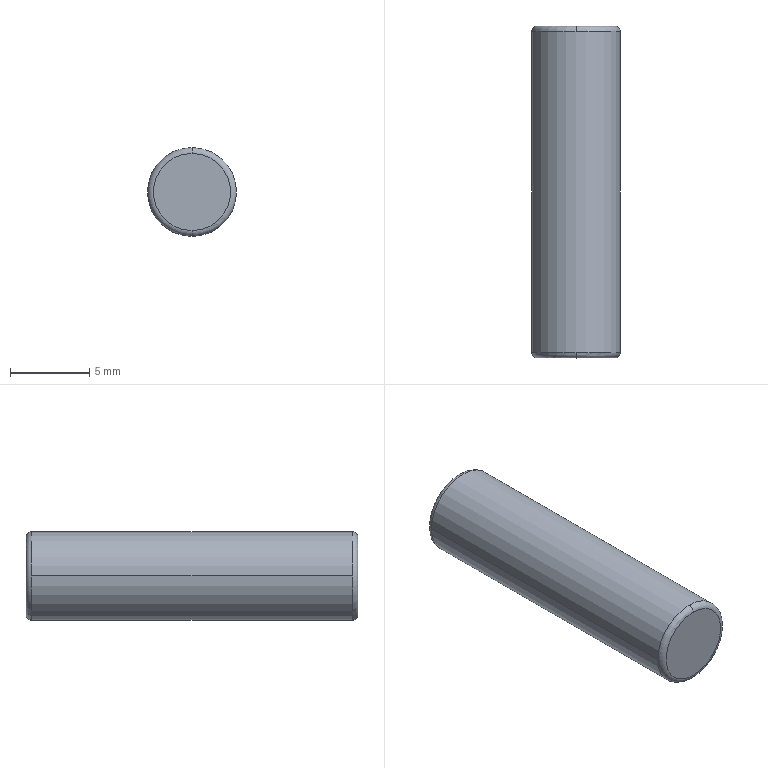Part | SolidWorks | features BaseBody 1 | 1 solid | 8 faces | box 5.625 x 21 x 5.625 mm | volume 520.859 mm3 | torus 4 | plane 2 | cylinder 2 | commonest cylinder face diameters 5.625 x2
STEP:
#1=CARTESIAN_POINT('',(-2092.012,757.069,-1580.068));
#2=VERTEX_POINT('',#1);
#3=CARTESIAN_POINT('',(-2092.012,757.069,-1575.181));
#4=VERTEX_POINT('',#3);
#5=CARTESIAN_POINT('',(-2092.012,757.069,-1577.624));
#6=DIRECTION('',(0.,-1.,0.));
#7=DIRECTION('',(1.,0.,0.));
#8=AXIS2_PLACEMENT_3D('',#5,#6,#7);
#9=CIRCLE('',#8,2.444);
#10=EDGE_CURVE('',#2,#4,#9,.T.);
#11=ORIENTED_EDGE('',*,*,#10,.T.);
#12=CARTESIAN_POINT('',(-2092.012,757.069,-1577.624));
#13=DIRECTION('',(0.,-1.,0.));
#14=DIRECTION('',(0.,0.,1.));
#15=AXIS2_PLACEMENT_3D('',#12,#13,#14);
#16=CIRCLE('',#15,2.444);
#17=EDGE_CURVE('',#4,#2,#16,.T.);
#18=ORIENTED_EDGE('',*,*,#17,.T.);
#19=EDGE_LOOP('',(#11,#18));
#20=FACE_OUTER_BOUND('',#19,.T.);
#21=CARTESIAN_POINT('',(-2094.675,757.069,-1580.313));
#22=DIRECTION('',(0.,-1.,0.));
#23=DIRECTION('',(0.,0.,-1.));
#24=AXIS2_PLACEMENT_3D('',#21,#22,#23);
#25=PLANE('',#24);
#26=ADVANCED_FACE('',(#20),#25,.T.);
#27=CARTESIAN_POINT('',(-2092.012,757.437,-1580.437));
#28=VERTEX_POINT('',#27);
#29=CARTESIAN_POINT('',(-2092.012,757.437,-1580.068));
#30=DIRECTION('',(-1.,0.,0.));
#31=DIRECTION('',(0.,0.,-1.));
#32=AXIS2_PLACEMENT_3D('',#29,#30,#31);
#33=CIRCLE('',#32,0.3687);
#34=EDGE_CURVE('',#28,#2,#33,.T.);
#35=ORIENTED_EDGE('',*,*,#34,.T.);
#36=ORIENTED_EDGE('',*,*,#17,.F.);
#37=CARTESIAN_POINT('',(-2092.012,757.437,-1574.812));
#38=VERTEX_POINT('',#37);
#39=CARTESIAN_POINT('',(-2092.012,757.437,-1575.181));
#40=DIRECTION('',(-1.,0.,0.));
#41=DIRECTION('',(0.,-1.,0.));
#42=AXIS2_PLACEMENT_3D('',#39,#40,#41);
#43=CIRCLE('',#42,0.3687);
#44=EDGE_CURVE('',#4,#38,#43,.T.);
#45=ORIENTED_EDGE('',*,*,#44,.T.);
#46=CARTESIAN_POINT('',(-2094.825,757.437,-1577.624));
#47=VERTEX_POINT('',#46);
#48=CARTESIAN_POINT('',(-2092.012,757.437,-1577.624));
#49=DIRECTION('',(0.,-1.,0.));
#50=DIRECTION('',(0.,0.,1.));
#51=AXIS2_PLACEMENT_3D('',#48,#49,#50);
#52=CIRCLE('',#51,2.813);
#53=EDGE_CURVE('',#38,#47,#52,.T.);
#54=ORIENTED_EDGE('',*,*,#53,.T.);
#55=CARTESIAN_POINT('',(-2092.012,757.437,-1577.624));
#56=DIRECTION('',(0.,-1.,0.));
#57=DIRECTION('',(-1.,0.,0.));
#58=AXIS2_PLACEMENT_3D('',#55,#56,#57);
#59=CIRCLE('',#58,2.813);
#60=EDGE_CURVE('',#47,#28,#59,.T.);
#61=ORIENTED_EDGE('',*,*,#60,.T.);
#62=EDGE_LOOP('',(#35,#36,#45,#54,#61));
#63=FACE_OUTER_BOUND('',#62,.T.);
#64=CARTESIAN_POINT('',(-2092.012,757.437,-1577.624));
#65=DIRECTION('',(0.,-1.,0.));
#66=DIRECTION('',(0.08716,0.,0.9962));
#67=AXIS2_PLACEMENT_3D('',#64,#65,#66);
#68=TOROIDAL_SURFACE('',#67,2.444,0.3687);
#69=ADVANCED_FACE('',(#63),#68,.T.);
#70=CARTESIAN_POINT('',(-2089.2,777.7,-1577.624));
#71=VERTEX_POINT('',#70);
#72=CARTESIAN_POINT('',(-2089.2,757.437,-1577.624));
#73=VERTEX_POINT('',#72);
#74=CARTESIAN_POINT('',(-2089.2,777.7,-1577.624));
#75=DIRECTION('',(0.,-1.,0.));
#76=VECTOR('',#75,1000.);
#77=LINE('',#74,#76);
#78=EDGE_CURVE('',#71,#73,#77,.T.);
#79=ORIENTED_EDGE('',*,*,#78,.T.);
#80=CARTESIAN_POINT('',(-2092.012,757.437,-1577.624));
#81=DIRECTION('',(0.,-1.,0.));
#82=DIRECTION('',(0.,0.,-1.));
#83=AXIS2_PLACEMENT_3D('',#80,#81,#82);
#84=CIRCLE('',#83,2.813);
#85=EDGE_CURVE('',#28,#73,#84,.T.);
#86=ORIENTED_EDGE('',*,*,#85,.F.);
#87=ORIENTED_EDGE('',*,*,#60,.F.);
#88=CARTESIAN_POINT('',(-2094.825,777.7,-1577.624));
#89=VERTEX_POINT('',#88);
#90=CARTESIAN_POINT('',(-2094.825,757.437,-1577.624));
#91=DIRECTION('',(0.,1.,0.));
#92=VECTOR('',#91,1000.);
#93=LINE('',#90,#92);
#94=EDGE_CURVE('',#47,#89,#93,.T.);
#95=ORIENTED_EDGE('',*,*,#94,.T.);
#96=CARTESIAN_POINT('',(-2092.012,777.7,-1580.437));
#97=VERTEX_POINT('',#96);
#98=CARTESIAN_POINT('',(-2092.012,777.7,-1577.624));
#99=DIRECTION('',(0.,-1.,0.));
#100=DIRECTION('',(-1.,0.,0.));
#101=AXIS2_PLACEMENT_3D('',#98,#99,#100);
#102=CIRCLE('',#101,2.813);
#103=EDGE_CURVE('',#89,#97,#102,.T.);
#104=ORIENTED_EDGE('',*,*,#103,.T.);
#105=CARTESIAN_POINT('',(-2092.012,777.7,-1577.624));
#106=DIRECTION('',(0.,-1.,0.));
#107=DIRECTION('',(0.,0.,-1.));
#108=AXIS2_PLACEMENT_3D('',#105,#106,#107);
#109=CIRCLE('',#108,2.813);
#110=EDGE_CURVE('',#97,#71,#109,.T.);
#111=ORIENTED_EDGE('',*,*,#110,.T.);
#112=EDGE_LOOP('',(#79,#86,#87,#95,#104,#111));
#113=FACE_OUTER_BOUND('',#112,.T.);
#114=CARTESIAN_POINT('',(-2092.012,778.713,-1577.624));
#115=DIRECTION('',(0.,1.,0.));
#116=DIRECTION('',(0.9962,0.,0.08716));
#117=AXIS2_PLACEMENT_3D('',#114,#115,#116);
#118=CYLINDRICAL_SURFACE('',#117,2.813);
#119=ADVANCED_FACE('',(#113),#118,.T.);
#120=CARTESIAN_POINT('',(-2092.012,778.069,-1580.068));
#121=VERTEX_POINT('',#120);
#122=CARTESIAN_POINT('',(-2092.012,777.7,-1580.068));
#123=DIRECTION('',(-1.,0.,0.));
#124=DIRECTION('',(0.,1.,0.));
#125=AXIS2_PLACEMENT_3D('',#122,#123,#124);
#126=CIRCLE('',#125,0.3687);
#127=EDGE_CURVE('',#121,#97,#126,.T.);
#128=ORIENTED_EDGE('',*,*,#127,.T.);
#129=ORIENTED_EDGE('',*,*,#103,.F.);
#130=CARTESIAN_POINT('',(-2092.012,777.7,-1574.812));
#131=VERTEX_POINT('',#130);
#132=CARTESIAN_POINT('',(-2092.012,777.7,-1577.624));
#133=DIRECTION('',(0.,-1.,0.));
#134=DIRECTION('',(0.,0.,1.));
#135=AXIS2_PLACEMENT_3D('',#132,#133,#134);
#136=CIRCLE('',#135,2.813);
#137=EDGE_CURVE('',#131,#89,#136,.T.);
#138=ORIENTED_EDGE('',*,*,#137,.F.);
#139=CARTESIAN_POINT('',(-2092.012,778.069,-1575.181));
#140=VERTEX_POINT('',#139);
#141=CARTESIAN_POINT('',(-2092.012,777.7,-1575.181));
#142=DIRECTION('',(-1.,0.,0.));
#143=DIRECTION('',(0.,0.,1.));
#144=AXIS2_PLACEMENT_3D('',#141,#142,#143);
#145=CIRCLE('',#144,0.3687);
#146=EDGE_CURVE('',#131,#140,#145,.T.);
#147=ORIENTED_EDGE('',*,*,#146,.T.);
#148=CARTESIAN_POINT('',(-2092.012,778.069,-1577.624));
#149=DIRECTION('',(0.,1.,0.));
#150=DIRECTION('',(0.,0.,-1.));
#151=AXIS2_PLACEMENT_3D('',#148,#149,#150);
#152=CIRCLE('',#151,2.444);
#153=EDGE_CURVE('',#121,#140,#152,.T.);
#154=ORIENTED_EDGE('',*,*,#153,.F.);
#155=EDGE_LOOP('',(#128,#129,#138,#147,#154));
#156=FACE_OUTER_BOUND('',#155,.T.);
#157=CARTESIAN_POINT('',(-2092.012,777.7,-1577.624));
#158=DIRECTION('',(0.,-1.,0.));
#159=DIRECTION('',(0.08716,0.,0.9962));
#160=AXIS2_PLACEMENT_3D('',#157,#158,#159);
#161=TOROIDAL_SURFACE('',#160,2.444,0.3687);
#162=ADVANCED_FACE('',(#156),#161,.T.);
#163=CARTESIAN_POINT('',(-2092.012,778.069,-1577.624));
#164=DIRECTION('',(0.,1.,0.));
#165=DIRECTION('',(0.,0.,1.));
#166=AXIS2_PLACEMENT_3D('',#163,#164,#165);
#167=CIRCLE('',#166,2.444);
#168=EDGE_CURVE('',#140,#121,#167,.T.);
#169=ORIENTED_EDGE('',*,*,#168,.T.);
#170=ORIENTED_EDGE('',*,*,#153,.T.);
#171=EDGE_LOOP('',(#169,#170));
#172=FACE_OUTER_BOUND('',#171,.T.);
#173=CARTESIAN_POINT('',(-2089.324,778.069,-1580.313));
#174=DIRECTION('',(0.,1.,0.));
#175=DIRECTION('',(1.,0.,0.));
#176=AXIS2_PLACEMENT_3D('',#173,#174,#175);
#177=PLANE('',#176);
#178=ADVANCED_FACE('',(#172),#177,.T.);
#179=ORIENTED_EDGE('',*,*,#127,.F.);
#180=ORIENTED_EDGE('',*,*,#168,.F.);
#181=ORIENTED_EDGE('',*,*,#146,.F.);
#182=CARTESIAN_POINT('',(-2092.012,777.7,-1577.624));
#183=DIRECTION('',(0.,-1.,0.));
#184=DIRECTION('',(1.,0.,0.));
#185=AXIS2_PLACEMENT_3D('',#182,#183,#184);
#186=CIRCLE('',#185,2.813);
#187=EDGE_CURVE('',#71,#131,#186,.T.);
#188=ORIENTED_EDGE('',*,*,#187,.F.);
#189=ORIENTED_EDGE('',*,*,#110,.F.);
#190=EDGE_LOOP('',(#179,#180,#181,#188,#189));
#191=FACE_OUTER_BOUND('',#190,.T.);
#192=CARTESIAN_POINT('',(-2092.012,777.7,-1577.624));
#193=DIRECTION('',(0.,-1.,0.));
#194=DIRECTION('',(-0.08716,0.,-0.9962));
#195=AXIS2_PLACEMENT_3D('',#192,#193,#194);
#196=TOROIDAL_SURFACE('',#195,2.444,0.3687);
#197=ADVANCED_FACE('',(#191),#196,.T.);
#198=ORIENTED_EDGE('',*,*,#78,.F.);
#199=ORIENTED_EDGE('',*,*,#187,.T.);
#200=ORIENTED_EDGE('',*,*,#137,.T.);
#201=ORIENTED_EDGE('',*,*,#94,.F.);
#202=ORIENTED_EDGE('',*,*,#53,.F.);
#203=CARTESIAN_POINT('',(-2092.012,757.437,-1577.624));
#204=DIRECTION('',(0.,-1.,0.));
#205=DIRECTION('',(1.,0.,0.));
#206=AXIS2_PLACEMENT_3D('',#203,#204,#205);
#207=CIRCLE('',#206,2.813);
#208=EDGE_CURVE('',#73,#38,#207,.T.);
#209=ORIENTED_EDGE('',*,*,#208,.F.);
#210=EDGE_LOOP('',(#198,#199,#200,#201,#202,#209));
#211=FACE_OUTER_BOUND('',#210,.T.);
#212=CARTESIAN_POINT('',(-2092.012,778.713,-1577.624));
#213=DIRECTION('',(0.,1.,0.));
#214=DIRECTION('',(-0.9962,0.,-0.08716));
#215=AXIS2_PLACEMENT_3D('',#212,#213,#214);
#216=CYLINDRICAL_SURFACE('',#215,2.813);
#217=ADVANCED_FACE('',(#211),#216,.T.);
#218=ORIENTED_EDGE('',*,*,#34,.F.);
#219=ORIENTED_EDGE('',*,*,#85,.T.);
#220=ORIENTED_EDGE('',*,*,#208,.T.);
#221=ORIENTED_EDGE('',*,*,#44,.F.);
#222=ORIENTED_EDGE('',*,*,#10,.F.);
#223=EDGE_LOOP('',(#218,#219,#220,#221,#222));
#224=FACE_OUTER_BOUND('',#223,.T.);
#225=CARTESIAN_POINT('',(-2092.012,757.437,-1577.624));
#226=DIRECTION('',(0.,-1.,0.));
#227=DIRECTION('',(-0.08716,0.,-0.9962));
#228=AXIS2_PLACEMENT_3D('',#225,#226,#227);
#229=TOROIDAL_SURFACE('',#228,2.444,0.3687);
#230=ADVANCED_FACE('',(#224),#229,.T.);
#231=CLOSED_SHELL('',(#26,#69,#119,#162,#178,#197,#217,#230));
#232=MANIFOLD_SOLID_BREP('',#231);
#233=CARTESIAN_POINT('',(0.,0.,0.));
#234=DIRECTION('',(0.,0.,1.));
#235=DIRECTION('',(1.,0.,0.));
#236=AXIS2_PLACEMENT_3D('',#233,#234,#235);
#237=(LENGTH_UNIT()NAMED_UNIT(*)SI_UNIT(.MILLI.,.METRE.));
#238=UNCERTAINTY_MEASURE_WITH_UNIT(LENGTH_MEASURE(0.00001),#237,'','');
#239=(NAMED_UNIT(*)PLANE_ANGLE_UNIT()SI_UNIT($,.RADIAN.));
#240=(NAMED_UNIT(*)SI_UNIT($,.STERADIAN.)SOLID_ANGLE_UNIT());
#241=(GEOMETRIC_REPRESENTATION_CONTEXT(3)GLOBAL_UNCERTAINTY_ASSIGNED_CONTEXT((#238))GLOBAL_UNIT_ASSIGNED_CONTEXT((#237,#239,#240))REPRESENTATION_CONTEXT('',''));
#242=ADVANCED_BREP_SHAPE_REPRESENTATION('',(#232,#236),#241);